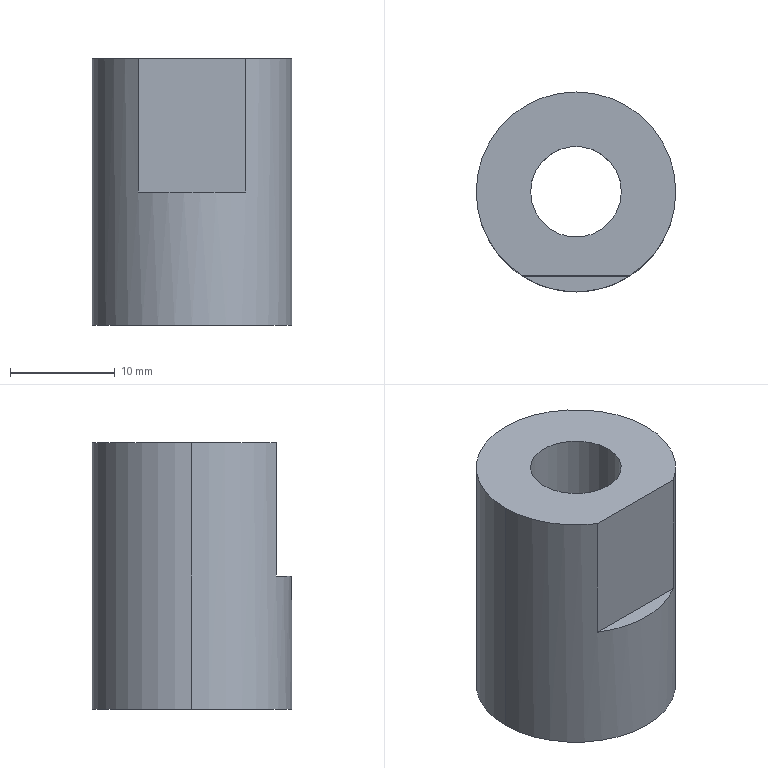Part | STEP file | 1_id1214_x_t | 1 solid | 10 faces | box 19.05 x 19.05 x 25.4 mm | volume 5054 mm3 | cylinder 5 | plane 5 | commonest cylinder face diameters 10.725 x2 19.05 x2 8.66 x1
STEP:
#1=CARTESIAN_POINT('',(0.,0.,0.));
#2=DIRECTION('',(0.,0.,1.));
#3=DIRECTION('',(1.,0.,0.));
#4=AXIS2_PLACEMENT_3D('',#1,#2,#3);
#5=CARTESIAN_POINT('',(145.14,175.234,-25.4));
#6=VERTEX_POINT('',#5);
#7=CARTESIAN_POINT('',(154.86,179.766,-25.4));
#8=VERTEX_POINT('',#7);
#9=CARTESIAN_POINT('',(150.,177.5,-25.4));
#10=DIRECTION('',(0.,0.,1.));
#11=DIRECTION('',(-0.9063,-0.4226,0.));
#12=AXIS2_PLACEMENT_3D('',#9,#10,#11);
#13=CIRCLE('',#12,5.362);
#14=CARTESIAN_POINT('',(150.,177.5,-45.));
#15=DIRECTION('',(0.,0.,1.));
#16=DIRECTION('',(0.9063,0.4226,0.));
#17=AXIS2_PLACEMENT_3D('',#14,#15,#16);
#18=CYLINDRICAL_SURFACE('',#17,5.362);
#19=CARTESIAN_POINT('',(3.142,19.6));
#20=DIRECTION('',(1.,0.));
#21=VECTOR('',#20,1.);
#22=LINE('',#19,#21);
#23=(GEOMETRIC_REPRESENTATION_CONTEXT(2)PARAMETRIC_REPRESENTATION_CONTEXT()REPRESENTATION_CONTEXT('',''));
#24=DEFINITIONAL_REPRESENTATION('',(#22),#23);
#25=PCURVE('',#18,#24);
#26=CARTESIAN_POINT('',(150.,177.5,-25.4));
#27=DIRECTION('',(0.,0.,1.));
#28=DIRECTION('',(0.9063,0.4226,0.));
#29=AXIS2_PLACEMENT_3D('',#26,#27,#28);
#30=PLANE('',#29);
#31=CARTESIAN_POINT('',(0.,0.));
#32=DIRECTION('',(-1.,0.));
#33=AXIS2_PLACEMENT_2D('',#31,#32);
#34=CIRCLE('',#33,5.362);
#35=(GEOMETRIC_REPRESENTATION_CONTEXT(2)PARAMETRIC_REPRESENTATION_CONTEXT()REPRESENTATION_CONTEXT('',''));
#36=DEFINITIONAL_REPRESENTATION('',(#34),#35);
#37=PCURVE('',#30,#36);
#38=SURFACE_CURVE('',#13,(#25,#37),.PCURVE_S1.);
#39=EDGE_CURVE('',#6,#8,#38,.T.);
#40=ORIENTED_EDGE('',*,*,#39,.T.);
#41=CARTESIAN_POINT('',(154.86,179.766,-7.7));
#42=VERTEX_POINT('',#41);
#43=CARTESIAN_POINT('',(154.86,179.766,-25.4));
#44=DIRECTION('',(0.,0.,1.));
#45=VECTOR('',#44,1.);
#46=LINE('',#43,#45);
#47=CARTESIAN_POINT('',(6.283,19.6));
#48=DIRECTION('',(0.,1.));
#49=VECTOR('',#48,1.);
#50=LINE('',#47,#49);
#51=(GEOMETRIC_REPRESENTATION_CONTEXT(2)PARAMETRIC_REPRESENTATION_CONTEXT()REPRESENTATION_CONTEXT('',''));
#52=DEFINITIONAL_REPRESENTATION('',(#50),#51);
#53=PCURVE('',#18,#52);
#54=CARTESIAN_POINT('',(150.,177.5,-45.));
#55=DIRECTION('',(0.,0.,1.));
#56=DIRECTION('',(0.9063,0.4226,0.));
#57=AXIS2_PLACEMENT_3D('',#54,#55,#56);
#58=CYLINDRICAL_SURFACE('',#57,5.362);
#59=CARTESIAN_POINT('',(0.,19.6));
#60=DIRECTION('',(0.,1.));
#61=VECTOR('',#60,1.);
#62=LINE('',#59,#61);
#63=(GEOMETRIC_REPRESENTATION_CONTEXT(2)PARAMETRIC_REPRESENTATION_CONTEXT()REPRESENTATION_CONTEXT('',''));
#64=DEFINITIONAL_REPRESENTATION('',(#62),#63);
#65=PCURVE('',#58,#64);
#66=SURFACE_CURVE('',#46,(#53,#65),.PCURVE_S1.);
#67=EDGE_CURVE('',#8,#42,#66,.T.);
#68=ORIENTED_EDGE('',*,*,#67,.T.);
#69=CARTESIAN_POINT('',(145.14,175.234,-7.7));
#70=VERTEX_POINT('',#69);
#71=CARTESIAN_POINT('',(150.,177.5,-7.7));
#72=DIRECTION('',(0.,0.,-1.));
#73=DIRECTION('',(0.9063,0.4226,0.));
#74=AXIS2_PLACEMENT_3D('',#71,#72,#73);
#75=CIRCLE('',#74,5.362);
#76=CARTESIAN_POINT('',(6.283,37.3));
#77=DIRECTION('',(-1.,0.));
#78=VECTOR('',#77,1.);
#79=LINE('',#76,#78);
#80=(GEOMETRIC_REPRESENTATION_CONTEXT(2)PARAMETRIC_REPRESENTATION_CONTEXT()REPRESENTATION_CONTEXT('',''));
#81=DEFINITIONAL_REPRESENTATION('',(#79),#80);
#82=PCURVE('',#18,#81);
#83=CARTESIAN_POINT('',(150.192,177.589,-7.7));
#84=DIRECTION('',(0.,0.,1.));
#85=DIRECTION('',(0.9063,0.4226,0.));
#86=AXIS2_PLACEMENT_3D('',#83,#84,#85);
#87=PLANE('',#86);
#88=CARTESIAN_POINT('',(5.151,0.));
#89=CARTESIAN_POINT('',(5.151,-9.288));
#90=CARTESIAN_POINT('',(-2.893,-4.644));
#91=CARTESIAN_POINT('',(-10.937,0.));
#92=CARTESIAN_POINT('',(-2.893,4.644));
#93=CARTESIAN_POINT('',(5.151,9.288));
#94=CARTESIAN_POINT('',(5.151,0.));
#95=(BOUNDED_CURVE()B_SPLINE_CURVE(2,(#88,#89,#90,#91,#92,#93,#94),.UNSPECIFIED.,.T.,.F.)B_SPLINE_CURVE_WITH_KNOTS((1,2,2,2,2,1),(-2.094,0.,2.094,4.189,6.283,8.378),.UNSPECIFIED.)CURVE()GEOMETRIC_REPRESENTATION_ITEM()RATIONAL_B_SPLINE_CURVE((1.,0.5,1.,0.5,1.,0.5,1.))REPRESENTATION_ITEM(''));
#96=(GEOMETRIC_REPRESENTATION_CONTEXT(2)PARAMETRIC_REPRESENTATION_CONTEXT()REPRESENTATION_CONTEXT('',''));
#97=DEFINITIONAL_REPRESENTATION('',(#95),#96);
#98=PCURVE('',#87,#97);
#99=SURFACE_CURVE('',#75,(#82,#98),.PCURVE_S1.);
#100=EDGE_CURVE('',#42,#70,#99,.T.);
#101=ORIENTED_EDGE('',*,*,#100,.T.);
#102=CARTESIAN_POINT('',(145.14,175.234,-25.4));
#103=DIRECTION('',(0.,0.,-1.));
#104=VECTOR('',#103,1.);
#105=LINE('',#102,#104);
#106=CARTESIAN_POINT('',(3.142,19.6));
#107=DIRECTION('',(0.,-1.));
#108=VECTOR('',#107,1.);
#109=LINE('',#106,#108);
#110=(GEOMETRIC_REPRESENTATION_CONTEXT(2)PARAMETRIC_REPRESENTATION_CONTEXT()REPRESENTATION_CONTEXT('',''));
#111=DEFINITIONAL_REPRESENTATION('',(#109),#110);
#112=PCURVE('',#18,#111);
#113=CARTESIAN_POINT('',(3.142,19.6));
#114=DIRECTION('',(0.,-1.));
#115=VECTOR('',#114,1.);
#116=LINE('',#113,#115);
#117=(GEOMETRIC_REPRESENTATION_CONTEXT(2)PARAMETRIC_REPRESENTATION_CONTEXT()REPRESENTATION_CONTEXT('',''));
#118=DEFINITIONAL_REPRESENTATION('',(#116),#117);
#119=PCURVE('',#58,#118);
#120=SURFACE_CURVE('',#105,(#112,#119),.PCURVE_S1.);
#121=EDGE_CURVE('',#70,#6,#120,.T.);
#122=ORIENTED_EDGE('',*,*,#121,.T.);
#123=EDGE_LOOP('',(#40,#68,#101,#122));
#124=FACE_BOUND('',#123,.F.);
#125=ADVANCED_FACE('',(#124),#18,.F.);
#126=CARTESIAN_POINT('',(159.525,177.5,-25.4));
#127=VERTEX_POINT('',#126);
#128=CARTESIAN_POINT('',(140.475,177.5,-25.4));
#129=VERTEX_POINT('',#128);
#130=CARTESIAN_POINT('',(150.,177.5,-25.4));
#131=DIRECTION('',(0.,0.,-1.));
#132=DIRECTION('',(1.,0.,0.));
#133=AXIS2_PLACEMENT_3D('',#130,#131,#132);
#134=CIRCLE('',#133,9.525);
#135=CARTESIAN_POINT('',(8.633,-4.025));
#136=CARTESIAN_POINT('',(1.66,-18.978));
#137=CARTESIAN_POINT('',(-7.802,-5.463));
#138=CARTESIAN_POINT('',(-17.265,8.051));
#139=CARTESIAN_POINT('',(-0.8302,9.489));
#140=CARTESIAN_POINT('',(15.605,10.927));
#141=CARTESIAN_POINT('',(8.633,-4.025));
#142=(BOUNDED_CURVE()B_SPLINE_CURVE(2,(#135,#136,#137,#138,#139,#140,#141),.UNSPECIFIED.,.T.,.F.)B_SPLINE_CURVE_WITH_KNOTS((1,2,2,2,2,1),(-2.094,0.,2.094,4.189,6.283,8.378),.UNSPECIFIED.)CURVE()GEOMETRIC_REPRESENTATION_ITEM()RATIONAL_B_SPLINE_CURVE((1.,0.5,1.,0.5,1.,0.5,1.))REPRESENTATION_ITEM(''));
#143=(GEOMETRIC_REPRESENTATION_CONTEXT(2)PARAMETRIC_REPRESENTATION_CONTEXT()REPRESENTATION_CONTEXT('',''));
#144=DEFINITIONAL_REPRESENTATION('',(#142),#143);
#145=PCURVE('',#30,#144);
#146=CARTESIAN_POINT('',(150.,177.5,-41.));
#147=DIRECTION('',(0.,0.,1.));
#148=DIRECTION('',(1.,0.,0.));
#149=AXIS2_PLACEMENT_3D('',#146,#147,#148);
#150=CYLINDRICAL_SURFACE('',#149,9.525);
#151=CARTESIAN_POINT('',(6.283,15.6));
#152=DIRECTION('',(-1.,0.));
#153=VECTOR('',#152,1.);
#154=LINE('',#151,#153);
#155=(GEOMETRIC_REPRESENTATION_CONTEXT(2)PARAMETRIC_REPRESENTATION_CONTEXT()REPRESENTATION_CONTEXT('',''));
#156=DEFINITIONAL_REPRESENTATION('',(#154),#155);
#157=PCURVE('',#150,#156);
#158=SURFACE_CURVE('',#134,(#145,#157),.PCURVE_S1.);
#159=EDGE_CURVE('',#127,#129,#158,.T.);
#160=ORIENTED_EDGE('',*,*,#159,.T.);
#161=CARTESIAN_POINT('',(150.,177.5,-25.4));
#162=DIRECTION('',(0.,0.,-1.));
#163=DIRECTION('',(-1.,0.,0.));
#164=AXIS2_PLACEMENT_3D('',#161,#162,#163);
#165=CIRCLE('',#164,9.525);
#166=CARTESIAN_POINT('',(-8.633,4.025));
#167=CARTESIAN_POINT('',(-1.66,18.978));
#168=CARTESIAN_POINT('',(7.802,5.463));
#169=CARTESIAN_POINT('',(17.265,-8.051));
#170=CARTESIAN_POINT('',(0.8302,-9.489));
#171=CARTESIAN_POINT('',(-15.605,-10.927));
#172=CARTESIAN_POINT('',(-8.633,4.025));
#173=(BOUNDED_CURVE()B_SPLINE_CURVE(2,(#166,#167,#168,#169,#170,#171,#172),.UNSPECIFIED.,.T.,.F.)B_SPLINE_CURVE_WITH_KNOTS((1,2,2,2,2,1),(-2.094,0.,2.094,4.189,6.283,8.378),.UNSPECIFIED.)CURVE()GEOMETRIC_REPRESENTATION_ITEM()RATIONAL_B_SPLINE_CURVE((1.,0.5,1.,0.5,1.,0.5,1.))REPRESENTATION_ITEM(''));
#174=(GEOMETRIC_REPRESENTATION_CONTEXT(2)PARAMETRIC_REPRESENTATION_CONTEXT()REPRESENTATION_CONTEXT('',''));
#175=DEFINITIONAL_REPRESENTATION('',(#173),#174);
#176=PCURVE('',#30,#175);
#177=CARTESIAN_POINT('',(150.,177.5,-41.));
#178=DIRECTION('',(0.,0.,1.));
#179=DIRECTION('',(1.,0.,0.));
#180=AXIS2_PLACEMENT_3D('',#177,#178,#179);
#181=CYLINDRICAL_SURFACE('',#180,9.525);
#182=CARTESIAN_POINT('',(3.142,15.6));
#183=DIRECTION('',(-1.,0.));
#184=VECTOR('',#183,1.);
#185=LINE('',#182,#184);
#186=(GEOMETRIC_REPRESENTATION_CONTEXT(2)PARAMETRIC_REPRESENTATION_CONTEXT()REPRESENTATION_CONTEXT('',''));
#187=DEFINITIONAL_REPRESENTATION('',(#185),#186);
#188=PCURVE('',#181,#187);
#189=SURFACE_CURVE('',#165,(#176,#188),.PCURVE_S1.);
#190=EDGE_CURVE('',#129,#127,#189,.T.);
#191=ORIENTED_EDGE('',*,*,#190,.T.);
#192=EDGE_LOOP('',(#160,#191));
#193=FACE_BOUND('',#192,.T.);
#194=CARTESIAN_POINT('',(150.,177.5,-25.4));
#195=DIRECTION('',(0.,0.,1.));
#196=DIRECTION('',(0.9063,0.4226,0.));
#197=AXIS2_PLACEMENT_3D('',#194,#195,#196);
#198=CIRCLE('',#197,5.362);
#199=CARTESIAN_POINT('',(0.,0.));
#200=DIRECTION('',(1.,0.));
#201=AXIS2_PLACEMENT_2D('',#199,#200);
#202=CIRCLE('',#201,5.362);
#203=(GEOMETRIC_REPRESENTATION_CONTEXT(2)PARAMETRIC_REPRESENTATION_CONTEXT()REPRESENTATION_CONTEXT('',''));
#204=DEFINITIONAL_REPRESENTATION('',(#202),#203);
#205=PCURVE('',#30,#204);
#206=CARTESIAN_POINT('',(0.,19.6));
#207=DIRECTION('',(1.,0.));
#208=VECTOR('',#207,1.);
#209=LINE('',#206,#208);
#210=(GEOMETRIC_REPRESENTATION_CONTEXT(2)PARAMETRIC_REPRESENTATION_CONTEXT()REPRESENTATION_CONTEXT('',''));
#211=DEFINITIONAL_REPRESENTATION('',(#209),#210);
#212=PCURVE('',#58,#211);
#213=SURFACE_CURVE('',#198,(#205,#212),.PCURVE_S1.);
#214=EDGE_CURVE('',#8,#6,#213,.T.);
#215=ORIENTED_EDGE('',*,*,#214,.T.);
#216=ORIENTED_EDGE('',*,*,#39,.T.);
#217=EDGE_LOOP('',(#215,#216));
#218=FACE_BOUND('',#217,.T.);
#219=ADVANCED_FACE('',(#193,#218),#30,.F.);
#220=ORIENTED_EDGE('',*,*,#214,.T.);
#221=ORIENTED_EDGE('',*,*,#121,.F.);
#222=CARTESIAN_POINT('',(150.,177.5,-7.7));
#223=DIRECTION('',(0.,0.,-1.));
#224=DIRECTION('',(-0.9063,-0.4226,0.));
#225=AXIS2_PLACEMENT_3D('',#222,#223,#224);
#226=CIRCLE('',#225,5.362);
#227=CARTESIAN_POINT('',(3.142,37.3));
#228=DIRECTION('',(-1.,0.));
#229=VECTOR('',#228,1.);
#230=LINE('',#227,#229);
#231=(GEOMETRIC_REPRESENTATION_CONTEXT(2)PARAMETRIC_REPRESENTATION_CONTEXT()REPRESENTATION_CONTEXT('',''));
#232=DEFINITIONAL_REPRESENTATION('',(#230),#231);
#233=PCURVE('',#58,#232);
#234=CARTESIAN_POINT('',(-5.574,0.));
#235=CARTESIAN_POINT('',(-5.574,9.288));
#236=CARTESIAN_POINT('',(2.47,4.644));
#237=CARTESIAN_POINT('',(10.513,0.));
#238=CARTESIAN_POINT('',(2.47,-4.644));
#239=CARTESIAN_POINT('',(-5.574,-9.288));
#240=CARTESIAN_POINT('',(-5.574,0.));
#241=(BOUNDED_CURVE()B_SPLINE_CURVE(2,(#234,#235,#236,#237,#238,#239,#240),.UNSPECIFIED.,.T.,.F.)B_SPLINE_CURVE_WITH_KNOTS((1,2,2,2,2,1),(-2.094,0.,2.094,4.189,6.283,8.378),.UNSPECIFIED.)CURVE()GEOMETRIC_REPRESENTATION_ITEM()RATIONAL_B_SPLINE_CURVE((1.,0.5,1.,0.5,1.,0.5,1.))REPRESENTATION_ITEM(''));
#242=(GEOMETRIC_REPRESENTATION_CONTEXT(2)PARAMETRIC_REPRESENTATION_CONTEXT()REPRESENTATION_CONTEXT('',''));
#243=DEFINITIONAL_REPRESENTATION('',(#241),#242);
#244=PCURVE('',#87,#243);
#245=SURFACE_CURVE('',#226,(#233,#244),.PCURVE_S1.);
#246=EDGE_CURVE('',#70,#42,#245,.T.);
#247=ORIENTED_EDGE('',*,*,#246,.T.);
#248=ORIENTED_EDGE('',*,*,#67,.F.);
#249=EDGE_LOOP('',(#220,#221,#247,#248));
#250=FACE_BOUND('',#249,.F.);
#251=ADVANCED_FACE('',(#250),#58,.F.);
#252=ORIENTED_EDGE('',*,*,#100,.T.);
#253=ORIENTED_EDGE('',*,*,#246,.T.);
#254=EDGE_LOOP('',(#252,#253));
#255=FACE_BOUND('',#254,.T.);
#256=CARTESIAN_POINT('',(154.33,177.5,-7.7));
#257=VERTEX_POINT('',#256);
#258=CARTESIAN_POINT('',(150.,177.5,-7.7));
#259=DIRECTION('',(0.,0.,1.));
#260=DIRECTION('',(1.,0.,0.));
#261=AXIS2_PLACEMENT_3D('',#258,#259,#260);
#262=CIRCLE('',#261,4.33);
#263=CARTESIAN_POINT('',(-0.2115,0.));
#264=DIRECTION('',(0.9063,-0.4226));
#265=AXIS2_PLACEMENT_2D('',#263,#264);
#266=CIRCLE('',#265,4.33);
#267=(GEOMETRIC_REPRESENTATION_CONTEXT(2)PARAMETRIC_REPRESENTATION_CONTEXT()REPRESENTATION_CONTEXT('',''));
#268=DEFINITIONAL_REPRESENTATION('',(#266),#267);
#269=PCURVE('',#87,#268);
#270=CARTESIAN_POINT('',(150.,177.5,-45.));
#271=DIRECTION('',(0.,0.,1.));
#272=DIRECTION('',(0.9063,0.4226,0.));
#273=AXIS2_PLACEMENT_3D('',#270,#271,#272);
#274=CYLINDRICAL_SURFACE('',#273,4.33);
#275=CARTESIAN_POINT('',(5.847,37.3));
#276=DIRECTION('',(1.,0.));
#277=VECTOR('',#276,1.);
#278=LINE('',#275,#277);
#279=(GEOMETRIC_REPRESENTATION_CONTEXT(2)PARAMETRIC_REPRESENTATION_CONTEXT()REPRESENTATION_CONTEXT('',''));
#280=DEFINITIONAL_REPRESENTATION('',(#278),#279);
#281=PCURVE('',#274,#280);
#282=SURFACE_CURVE('',#262,(#269,#281),.PCURVE_S1.);
#283=EDGE_CURVE('',#257,#257,#282,.T.);
#284=ORIENTED_EDGE('',*,*,#283,.T.);
#285=EDGE_LOOP('',(#284));
#286=FACE_BOUND('',#285,.T.);
#287=ADVANCED_FACE('',(#255,#286),#87,.F.);
#288=CARTESIAN_POINT('',(144.869,169.475,0.));
#289=VERTEX_POINT('',#288);
#290=CARTESIAN_POINT('',(155.131,169.475,0.));
#291=VERTEX_POINT('',#290);
#292=CARTESIAN_POINT('',(144.869,169.475,0.));
#293=DIRECTION('',(1.,0.,0.));
#294=VECTOR('',#293,1.);
#295=LINE('',#292,#294);
#296=CARTESIAN_POINT('',(150.,177.5,0.));
#297=DIRECTION('',(0.,0.,1.));
#298=DIRECTION('',(0.9063,0.4226,0.));
#299=AXIS2_PLACEMENT_3D('',#296,#297,#298);
#300=PLANE('',#299);
#301=CARTESIAN_POINT('',(-8.042,-5.105));
#302=DIRECTION('',(0.9063,-0.4226));
#303=VECTOR('',#302,1.);
#304=LINE('',#301,#303);
#305=(GEOMETRIC_REPRESENTATION_CONTEXT(2)PARAMETRIC_REPRESENTATION_CONTEXT()REPRESENTATION_CONTEXT('',''));
#306=DEFINITIONAL_REPRESENTATION('',(#304),#305);
#307=PCURVE('',#300,#306);
#308=CARTESIAN_POINT('',(154.617,169.475,-9.5));
#309=DIRECTION('',(0.,-1.,0.));
#310=DIRECTION('',(0.,0.,1.));
#311=AXIS2_PLACEMENT_3D('',#308,#309,#310);
#312=PLANE('',#311);
#313=CARTESIAN_POINT('',(9.5,9.748));
#314=DIRECTION('',(0.,-1.));
#315=VECTOR('',#314,1.);
#316=LINE('',#313,#315);
#317=(GEOMETRIC_REPRESENTATION_CONTEXT(2)PARAMETRIC_REPRESENTATION_CONTEXT()REPRESENTATION_CONTEXT('',''));
#318=DEFINITIONAL_REPRESENTATION('',(#316),#317);
#319=PCURVE('',#312,#318);
#320=SURFACE_CURVE('',#295,(#307,#319),.PCURVE_S1.);
#321=EDGE_CURVE('',#289,#291,#320,.T.);
#322=ORIENTED_EDGE('',*,*,#321,.T.);
#323=CARTESIAN_POINT('',(159.525,177.5,0.));
#324=VERTEX_POINT('',#323);
#325=CARTESIAN_POINT('',(150.,177.5,0.));
#326=DIRECTION('',(0.,0.,1.));
#327=DIRECTION('',(0.5387,-0.8425,0.));
#328=AXIS2_PLACEMENT_3D('',#325,#326,#327);
#329=CIRCLE('',#328,9.525);
#330=CARTESIAN_POINT('',(0.,0.));
#331=DIRECTION('',(0.1321,-0.9912));
#332=AXIS2_PLACEMENT_2D('',#330,#331);
#333=CIRCLE('',#332,9.525);
#334=(GEOMETRIC_REPRESENTATION_CONTEXT(2)PARAMETRIC_REPRESENTATION_CONTEXT()REPRESENTATION_CONTEXT('',''));
#335=DEFINITIONAL_REPRESENTATION('',(#333),#334);
#336=PCURVE('',#300,#335);
#337=CARTESIAN_POINT('',(5.281,41.));
#338=DIRECTION('',(1.,0.));
#339=VECTOR('',#338,1.);
#340=LINE('',#337,#339);
#341=(GEOMETRIC_REPRESENTATION_CONTEXT(2)PARAMETRIC_REPRESENTATION_CONTEXT()REPRESENTATION_CONTEXT('',''));
#342=DEFINITIONAL_REPRESENTATION('',(#340),#341);
#343=PCURVE('',#150,#342);
#344=SURFACE_CURVE('',#329,(#336,#343),.PCURVE_S1.);
#345=EDGE_CURVE('',#291,#324,#344,.T.);
#346=ORIENTED_EDGE('',*,*,#345,.T.);
#347=CARTESIAN_POINT('',(140.475,177.5,0.));
#348=VERTEX_POINT('',#347);
#349=CARTESIAN_POINT('',(150.,177.5,0.));
#350=DIRECTION('',(0.,0.,1.));
#351=DIRECTION('',(1.,0.,0.));
#352=AXIS2_PLACEMENT_3D('',#349,#350,#351);
#353=CIRCLE('',#352,9.525);
#354=CARTESIAN_POINT('',(0.,0.));
#355=DIRECTION('',(0.9063,-0.4226));
#356=AXIS2_PLACEMENT_2D('',#354,#355);
#357=CIRCLE('',#356,9.525);
#358=(GEOMETRIC_REPRESENTATION_CONTEXT(2)PARAMETRIC_REPRESENTATION_CONTEXT()REPRESENTATION_CONTEXT('',''));
#359=DEFINITIONAL_REPRESENTATION('',(#357),#358);
#360=PCURVE('',#300,#359);
#361=CARTESIAN_POINT('',(0.,41.));
#362=DIRECTION('',(1.,0.));
#363=VECTOR('',#362,1.);
#364=LINE('',#361,#363);
#365=(GEOMETRIC_REPRESENTATION_CONTEXT(2)PARAMETRIC_REPRESENTATION_CONTEXT()REPRESENTATION_CONTEXT('',''));
#366=DEFINITIONAL_REPRESENTATION('',(#364),#365);
#367=PCURVE('',#181,#366);
#368=SURFACE_CURVE('',#353,(#360,#367),.PCURVE_S1.);
#369=EDGE_CURVE('',#324,#348,#368,.T.);
#370=ORIENTED_EDGE('',*,*,#369,.T.);
#371=CARTESIAN_POINT('',(150.,177.5,0.));
#372=DIRECTION('',(0.,0.,1.));
#373=DIRECTION('',(-1.,0.000000006,0.));
#374=AXIS2_PLACEMENT_3D('',#371,#372,#373);
#375=CIRCLE('',#374,9.525);
#376=CARTESIAN_POINT('',(0.,0.));
#377=DIRECTION('',(-0.9063,0.4226));
#378=AXIS2_PLACEMENT_2D('',#376,#377);
#379=CIRCLE('',#378,9.525);
#380=(GEOMETRIC_REPRESENTATION_CONTEXT(2)PARAMETRIC_REPRESENTATION_CONTEXT()REPRESENTATION_CONTEXT('',''));
#381=DEFINITIONAL_REPRESENTATION('',(#379),#380);
#382=PCURVE('',#300,#381);
#383=CARTESIAN_POINT('',(3.142,41.));
#384=DIRECTION('',(1.,0.));
#385=VECTOR('',#384,1.);
#386=LINE('',#383,#385);
#387=(GEOMETRIC_REPRESENTATION_CONTEXT(2)PARAMETRIC_REPRESENTATION_CONTEXT()REPRESENTATION_CONTEXT('',''));
#388=DEFINITIONAL_REPRESENTATION('',(#386),#387);
#389=PCURVE('',#150,#388);
#390=SURFACE_CURVE('',#375,(#382,#389),.PCURVE_S1.);
#391=EDGE_CURVE('',#348,#289,#390,.T.);
#392=ORIENTED_EDGE('',*,*,#391,.T.);
#393=EDGE_LOOP('',(#322,#346,#370,#392));
#394=FACE_BOUND('',#393,.T.);
#395=CARTESIAN_POINT('',(154.33,177.5,0.));
#396=VERTEX_POINT('',#395);
#397=CARTESIAN_POINT('',(150.,177.5,0.));
#398=DIRECTION('',(0.,0.,-1.));
#399=DIRECTION('',(1.,0.,0.));
#400=AXIS2_PLACEMENT_3D('',#397,#398,#399);
#401=CIRCLE('',#400,4.33);
#402=CARTESIAN_POINT('',(3.924,-1.83));
#403=CARTESIAN_POINT('',(0.7548,-8.627));
#404=CARTESIAN_POINT('',(-3.547,-2.484));
#405=CARTESIAN_POINT('',(-7.849,3.66));
#406=CARTESIAN_POINT('',(-0.3774,4.314));
#407=CARTESIAN_POINT('',(7.094,4.967));
#408=CARTESIAN_POINT('',(3.924,-1.83));
#409=(BOUNDED_CURVE()B_SPLINE_CURVE(2,(#402,#403,#404,#405,#406,#407,#408),.UNSPECIFIED.,.T.,.F.)B_SPLINE_CURVE_WITH_KNOTS((1,2,2,2,2,1),(-2.094,0.,2.094,4.189,6.283,8.378),.UNSPECIFIED.)CURVE()GEOMETRIC_REPRESENTATION_ITEM()RATIONAL_B_SPLINE_CURVE((1.,0.5,1.,0.5,1.,0.5,1.))REPRESENTATION_ITEM(''));
#410=(GEOMETRIC_REPRESENTATION_CONTEXT(2)PARAMETRIC_REPRESENTATION_CONTEXT()REPRESENTATION_CONTEXT('',''));
#411=DEFINITIONAL_REPRESENTATION('',(#409),#410);
#412=PCURVE('',#300,#411);
#413=CARTESIAN_POINT('',(12.13,45.));
#414=DIRECTION('',(-1.,0.));
#415=VECTOR('',#414,1.);
#416=LINE('',#413,#415);
#417=(GEOMETRIC_REPRESENTATION_CONTEXT(2)PARAMETRIC_REPRESENTATION_CONTEXT()REPRESENTATION_CONTEXT('',''));
#418=DEFINITIONAL_REPRESENTATION('',(#416),#417);
#419=PCURVE('',#274,#418);
#420=SURFACE_CURVE('',#401,(#412,#419),.PCURVE_S1.);
#421=EDGE_CURVE('',#396,#396,#420,.T.);
#422=ORIENTED_EDGE('',*,*,#421,.T.);
#423=EDGE_LOOP('',(#422));
#424=FACE_BOUND('',#423,.T.);
#425=ADVANCED_FACE('',(#394,#424),#300,.T.);
#426=ORIENTED_EDGE('',*,*,#421,.T.);
#427=CARTESIAN_POINT('',(154.33,177.5,-7.7));
#428=CARTESIAN_POINT('',(154.33,177.5,0.));
#429=B_SPLINE_CURVE_WITH_KNOTS('',1,(#427,#428),.UNSPECIFIED.,.F.,.F.,(2,2),(37.3,45.),.PIECEWISE_BEZIER_KNOTS.);
#430=CARTESIAN_POINT('',(5.847,0.));
#431=DIRECTION('',(0.,1.));
#432=VECTOR('',#431,1.);
#433=LINE('',#430,#432);
#434=(GEOMETRIC_REPRESENTATION_CONTEXT(2)PARAMETRIC_REPRESENTATION_CONTEXT()REPRESENTATION_CONTEXT('',''));
#435=DEFINITIONAL_REPRESENTATION('',(#433),#434);
#436=PCURVE('',#274,#435);
#437=CARTESIAN_POINT('',(12.13,0.));
#438=DIRECTION('',(0.,1.));
#439=VECTOR('',#438,1.);
#440=LINE('',#437,#439);
#441=(GEOMETRIC_REPRESENTATION_CONTEXT(2)PARAMETRIC_REPRESENTATION_CONTEXT()REPRESENTATION_CONTEXT('',''));
#442=DEFINITIONAL_REPRESENTATION('',(#440),#441);
#443=PCURVE('',#274,#442);
#444=SEAM_CURVE('',#429,(#436,#443),.PCURVE_S1.);
#445=EDGE_CURVE('',#257,#396,#444,.T.);
#446=ORIENTED_EDGE('',*,*,#445,.F.);
#447=ORIENTED_EDGE('',*,*,#283,.T.);
#448=ORIENTED_EDGE('',*,*,#445,.T.);
#449=EDGE_LOOP('',(#426,#446,#447,#448));
#450=FACE_BOUND('',#449,.F.);
#451=ADVANCED_FACE('',(#450),#274,.F.);
#452=CARTESIAN_POINT('',(159.525,177.5,-25.4));
#453=DIRECTION('',(0.,0.,-1.));
#454=VECTOR('',#453,1.);
#455=LINE('',#452,#454);
#456=CARTESIAN_POINT('',(6.283,15.6));
#457=DIRECTION('',(0.,-1.));
#458=VECTOR('',#457,1.);
#459=LINE('',#456,#458);
#460=(GEOMETRIC_REPRESENTATION_CONTEXT(2)PARAMETRIC_REPRESENTATION_CONTEXT()REPRESENTATION_CONTEXT('',''));
#461=DEFINITIONAL_REPRESENTATION('',(#459),#460);
#462=PCURVE('',#150,#461);
#463=CARTESIAN_POINT('',(0.,15.6));
#464=DIRECTION('',(0.,-1.));
#465=VECTOR('',#464,1.);
#466=LINE('',#463,#465);
#467=(GEOMETRIC_REPRESENTATION_CONTEXT(2)PARAMETRIC_REPRESENTATION_CONTEXT()REPRESENTATION_CONTEXT('',''));
#468=DEFINITIONAL_REPRESENTATION('',(#466),#467);
#469=PCURVE('',#181,#468);
#470=SURFACE_CURVE('',#455,(#462,#469),.PCURVE_S1.);
#471=EDGE_CURVE('',#324,#127,#470,.T.);
#472=ORIENTED_EDGE('',*,*,#471,.F.);
#473=ORIENTED_EDGE('',*,*,#345,.F.);
#474=CARTESIAN_POINT('',(155.131,169.475,-12.7));
#475=VERTEX_POINT('',#474);
#476=CARTESIAN_POINT('',(155.131,169.475,0.));
#477=DIRECTION('',(0.,0.,-1.));
#478=VECTOR('',#477,1.);
#479=LINE('',#476,#478);
#480=CARTESIAN_POINT('',(5.281,41.));
#481=DIRECTION('',(0.,-1.));
#482=VECTOR('',#481,1.);
#483=LINE('',#480,#482);
#484=(GEOMETRIC_REPRESENTATION_CONTEXT(2)PARAMETRIC_REPRESENTATION_CONTEXT()REPRESENTATION_CONTEXT('',''));
#485=DEFINITIONAL_REPRESENTATION('',(#483),#484);
#486=PCURVE('',#150,#485);
#487=CARTESIAN_POINT('',(9.5,-0.514));
#488=DIRECTION('',(-1.,0.));
#489=VECTOR('',#488,1.);
#490=LINE('',#487,#489);
#491=(GEOMETRIC_REPRESENTATION_CONTEXT(2)PARAMETRIC_REPRESENTATION_CONTEXT()REPRESENTATION_CONTEXT('',''));
#492=DEFINITIONAL_REPRESENTATION('',(#490),#491);
#493=PCURVE('',#312,#492);
#494=SURFACE_CURVE('',#479,(#486,#493),.PCURVE_S1.);
#495=EDGE_CURVE('',#291,#475,#494,.T.);
#496=ORIENTED_EDGE('',*,*,#495,.T.);
#497=CARTESIAN_POINT('',(144.869,169.475,-12.7));
#498=VERTEX_POINT('',#497);
#499=CARTESIAN_POINT('',(150.,177.5,-12.7));
#500=DIRECTION('',(0.,0.,1.));
#501=DIRECTION('',(-0.5387,-0.8425,0.));
#502=AXIS2_PLACEMENT_3D('',#499,#500,#501);
#503=CIRCLE('',#502,9.525);
#504=CARTESIAN_POINT('',(4.144,28.3));
#505=DIRECTION('',(1.,0.));
#506=VECTOR('',#505,1.);
#507=LINE('',#504,#506);
#508=(GEOMETRIC_REPRESENTATION_CONTEXT(2)PARAMETRIC_REPRESENTATION_CONTEXT()REPRESENTATION_CONTEXT('',''));
#509=DEFINITIONAL_REPRESENTATION('',(#507),#508);
#510=PCURVE('',#150,#509);
#511=CARTESIAN_POINT('',(150.,177.5,-12.7));
#512=DIRECTION('',(0.,0.,1.));
#513=DIRECTION('',(0.9063,0.4226,0.));
#514=AXIS2_PLACEMENT_3D('',#511,#512,#513);
#515=PLANE('',#514);
#516=CARTESIAN_POINT('',(0.,0.));
#517=DIRECTION('',(-0.8443,-0.5359));
#518=AXIS2_PLACEMENT_2D('',#516,#517);
#519=CIRCLE('',#518,9.525);
#520=(GEOMETRIC_REPRESENTATION_CONTEXT(2)PARAMETRIC_REPRESENTATION_CONTEXT()REPRESENTATION_CONTEXT('',''));
#521=DEFINITIONAL_REPRESENTATION('',(#519),#520);
#522=PCURVE('',#515,#521);
#523=SURFACE_CURVE('',#503,(#510,#522),.PCURVE_S1.);
#524=EDGE_CURVE('',#498,#475,#523,.T.);
#525=ORIENTED_EDGE('',*,*,#524,.F.);
#526=CARTESIAN_POINT('',(144.869,169.475,-12.7));
#527=DIRECTION('',(0.,0.,1.));
#528=VECTOR('',#527,1.);
#529=LINE('',#526,#528);
#530=CARTESIAN_POINT('',(4.144,28.3));
#531=DIRECTION('',(0.,1.));
#532=VECTOR('',#531,1.);
#533=LINE('',#530,#532);
#534=(GEOMETRIC_REPRESENTATION_CONTEXT(2)PARAMETRIC_REPRESENTATION_CONTEXT()REPRESENTATION_CONTEXT('',''));
#535=DEFINITIONAL_REPRESENTATION('',(#533),#534);
#536=PCURVE('',#150,#535);
#537=CARTESIAN_POINT('',(-3.2,9.748));
#538=DIRECTION('',(1.,0.));
#539=VECTOR('',#538,1.);
#540=LINE('',#537,#539);
#541=(GEOMETRIC_REPRESENTATION_CONTEXT(2)PARAMETRIC_REPRESENTATION_CONTEXT()REPRESENTATION_CONTEXT('',''));
#542=DEFINITIONAL_REPRESENTATION('',(#540),#541);
#543=PCURVE('',#312,#542);
#544=SURFACE_CURVE('',#529,(#536,#543),.PCURVE_S1.);
#545=EDGE_CURVE('',#498,#289,#544,.T.);
#546=ORIENTED_EDGE('',*,*,#545,.T.);
#547=ORIENTED_EDGE('',*,*,#391,.F.);
#548=CARTESIAN_POINT('',(140.475,177.5,-41.));
#549=DIRECTION('',(0.,0.,1.));
#550=VECTOR('',#549,1.);
#551=LINE('',#548,#550);
#552=CARTESIAN_POINT('',(3.142,0.));
#553=DIRECTION('',(0.,1.));
#554=VECTOR('',#553,1.);
#555=LINE('',#552,#554);
#556=(GEOMETRIC_REPRESENTATION_CONTEXT(2)PARAMETRIC_REPRESENTATION_CONTEXT()REPRESENTATION_CONTEXT('',''));
#557=DEFINITIONAL_REPRESENTATION('',(#555),#556);
#558=PCURVE('',#150,#557);
#559=CARTESIAN_POINT('',(3.142,0.));
#560=DIRECTION('',(0.,1.));
#561=VECTOR('',#560,1.);
#562=LINE('',#559,#561);
#563=(GEOMETRIC_REPRESENTATION_CONTEXT(2)PARAMETRIC_REPRESENTATION_CONTEXT()REPRESENTATION_CONTEXT('',''));
#564=DEFINITIONAL_REPRESENTATION('',(#562),#563);
#565=PCURVE('',#181,#564);
#566=SURFACE_CURVE('',#551,(#558,#565),.PCURVE_S1.);
#567=EDGE_CURVE('',#129,#348,#566,.T.);
#568=ORIENTED_EDGE('',*,*,#567,.F.);
#569=ORIENTED_EDGE('',*,*,#159,.F.);
#570=EDGE_LOOP('',(#472,#473,#496,#525,#546,#547,#568,#569));
#571=FACE_BOUND('',#570,.T.);
#572=ADVANCED_FACE('',(#571),#150,.T.);
#573=ORIENTED_EDGE('',*,*,#567,.T.);
#574=ORIENTED_EDGE('',*,*,#369,.F.);
#575=ORIENTED_EDGE('',*,*,#471,.T.);
#576=ORIENTED_EDGE('',*,*,#190,.F.);
#577=EDGE_LOOP('',(#573,#574,#575,#576));
#578=FACE_BOUND('',#577,.T.);
#579=ADVANCED_FACE('',(#578),#181,.T.);
#580=CARTESIAN_POINT('',(155.131,169.475,-12.7));
#581=DIRECTION('',(-1.,0.,0.));
#582=VECTOR('',#581,1.);
#583=LINE('',#580,#582);
#584=CARTESIAN_POINT('',(-3.2,-0.514));
#585=DIRECTION('',(0.,1.));
#586=VECTOR('',#585,1.);
#587=LINE('',#584,#586);
#588=(GEOMETRIC_REPRESENTATION_CONTEXT(2)PARAMETRIC_REPRESENTATION_CONTEXT()REPRESENTATION_CONTEXT('',''));
#589=DEFINITIONAL_REPRESENTATION('',(#587),#588);
#590=PCURVE('',#312,#589);
#591=CARTESIAN_POINT('',(1.259,-9.441));
#592=DIRECTION('',(-0.9063,0.4226));
#593=VECTOR('',#592,1.);
#594=LINE('',#591,#593);
#595=(GEOMETRIC_REPRESENTATION_CONTEXT(2)PARAMETRIC_REPRESENTATION_CONTEXT()REPRESENTATION_CONTEXT('',''));
#596=DEFINITIONAL_REPRESENTATION('',(#594),#595);
#597=PCURVE('',#515,#596);
#598=SURFACE_CURVE('',#583,(#590,#597),.PCURVE_S1.);
#599=EDGE_CURVE('',#475,#498,#598,.T.);
#600=ORIENTED_EDGE('',*,*,#599,.F.);
#601=ORIENTED_EDGE('',*,*,#495,.F.);
#602=ORIENTED_EDGE('',*,*,#321,.F.);
#603=ORIENTED_EDGE('',*,*,#545,.F.);
#604=EDGE_LOOP('',(#600,#601,#602,#603));
#605=FACE_BOUND('',#604,.T.);
#606=ADVANCED_FACE('',(#605),#312,.T.);
#607=ORIENTED_EDGE('',*,*,#524,.T.);
#608=ORIENTED_EDGE('',*,*,#599,.T.);
#609=EDGE_LOOP('',(#607,#608));
#610=FACE_BOUND('',#609,.T.);
#611=ADVANCED_FACE('',(#610),#515,.T.);
#612=CLOSED_SHELL('',(#125,#219,#251,#287,#425,#451,#572,#579,#606,#611));
#613=MANIFOLD_SOLID_BREP('',#612);
#614=(LENGTH_UNIT()NAMED_UNIT(*)SI_UNIT(.MILLI.,.METRE.));
#615=UNCERTAINTY_MEASURE_WITH_UNIT(LENGTH_MEASURE(0.000001),#614,'','');
#616=(NAMED_UNIT(*)PLANE_ANGLE_UNIT()SI_UNIT($,.RADIAN.));
#617=(NAMED_UNIT(*)SI_UNIT($,.STERADIAN.)SOLID_ANGLE_UNIT());
#618=(GEOMETRIC_REPRESENTATION_CONTEXT(3)GLOBAL_UNCERTAINTY_ASSIGNED_CONTEXT((#615))GLOBAL_UNIT_ASSIGNED_CONTEXT((#614,#616,#617))REPRESENTATION_CONTEXT('',''));
#619=ADVANCED_BREP_SHAPE_REPRESENTATION('',(#4,#613),#618);